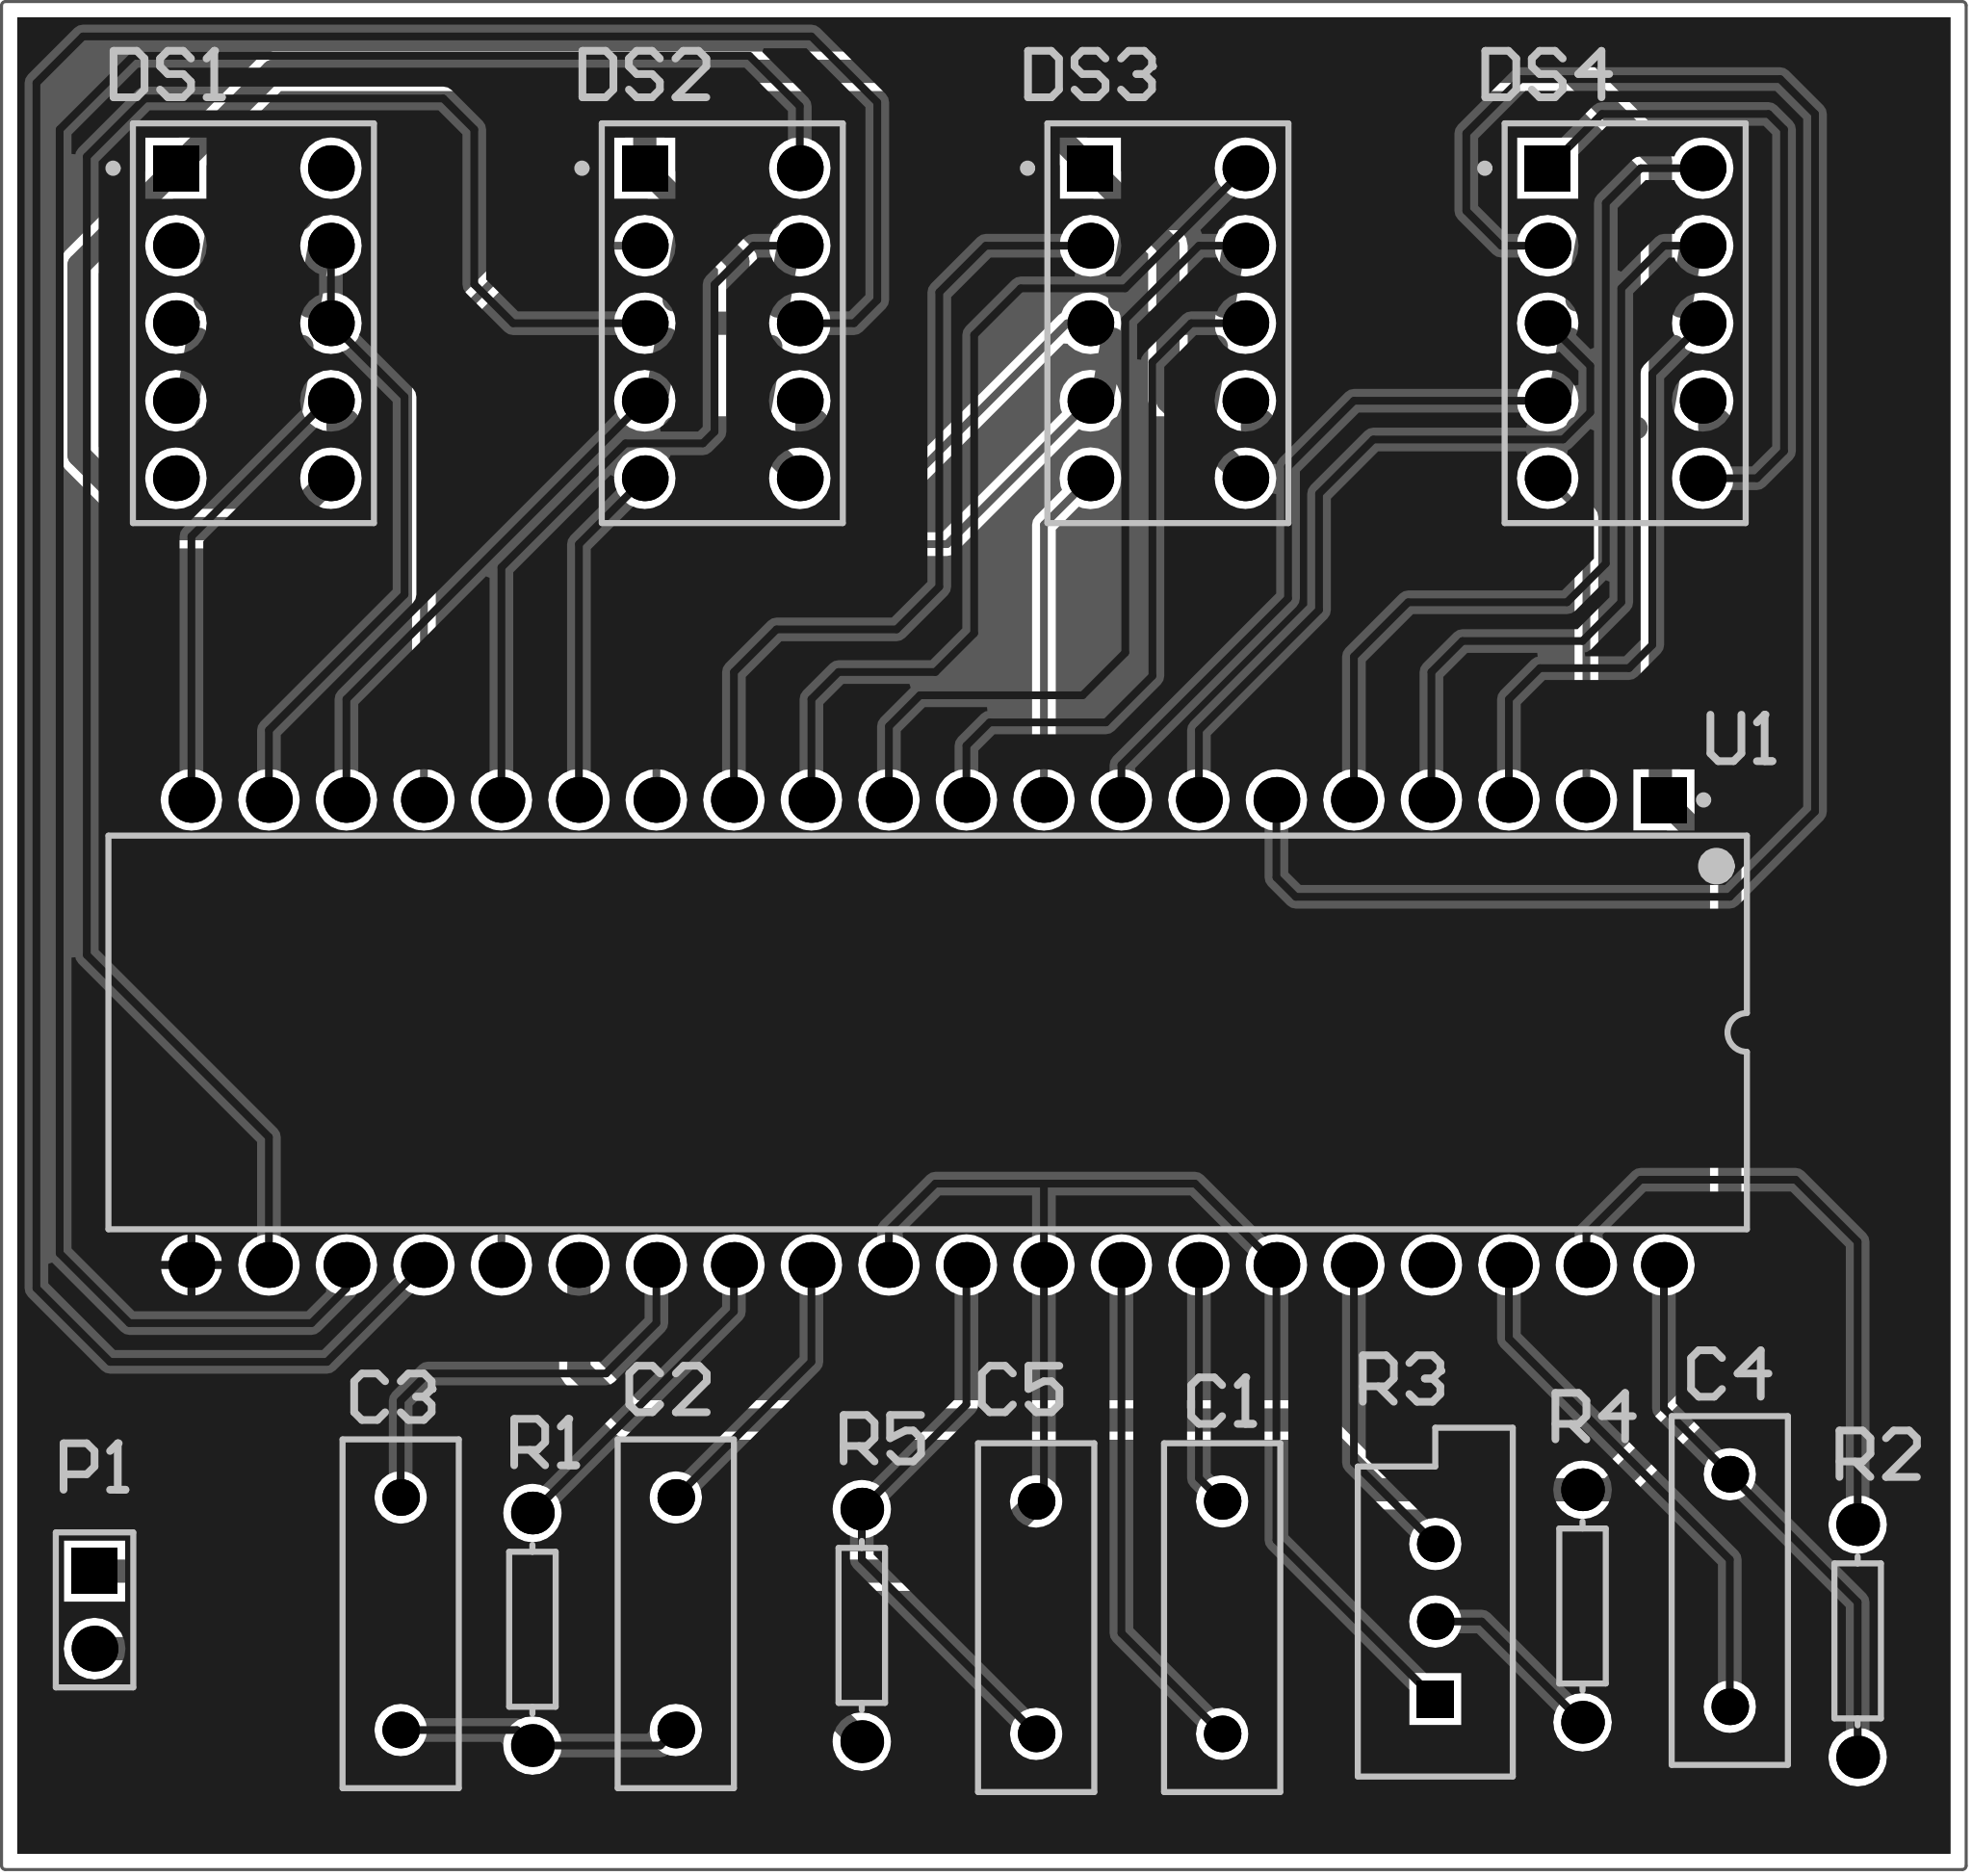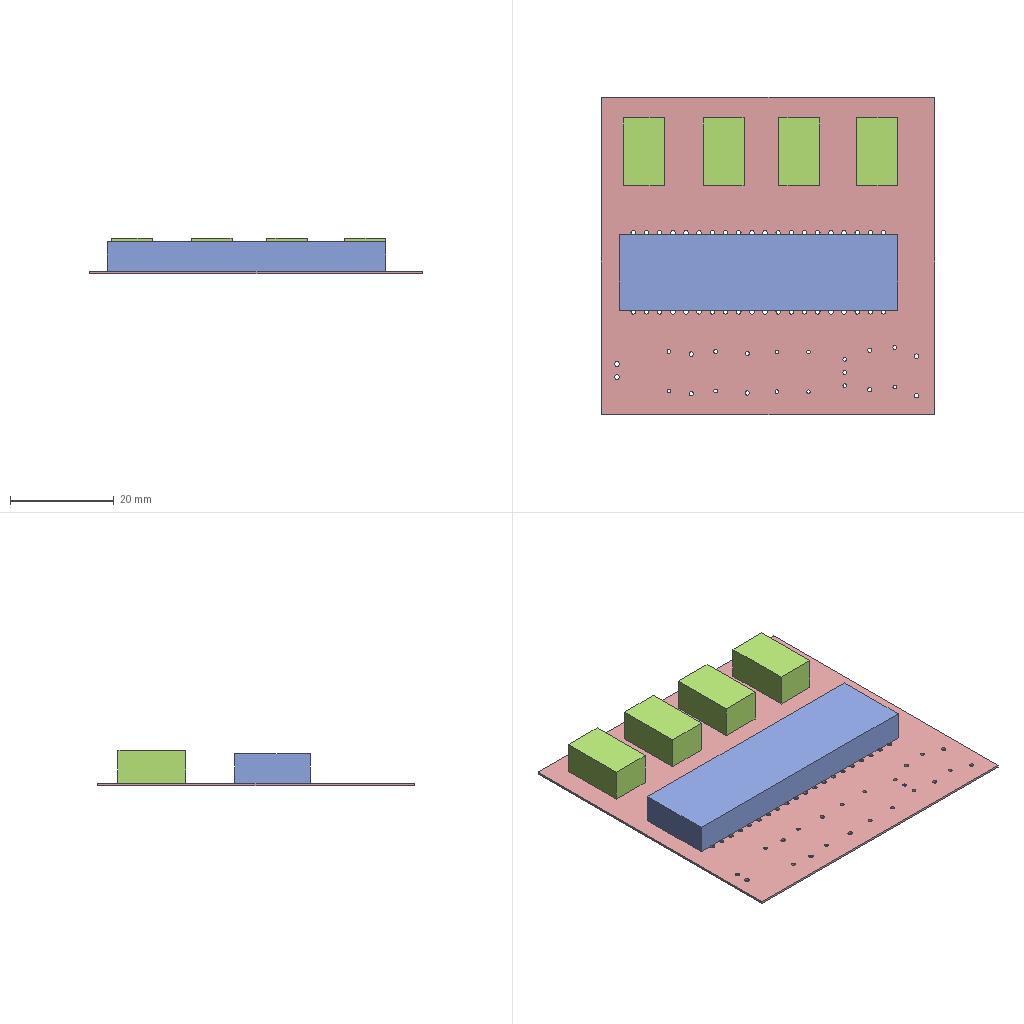Circuit board layout | Altium Designer | box 64.4 x 61.2 x 6.8 mm
Layer stack:
# Altium Designer layer stack of  (unit mm; dielectric type: 0 none, 1 core, 2 prepreg, 3 surface material)
index,name,kind,layer,copper_thickness_mm,dielectric_type,dielectric_thickness_mm,dielectric_material,dielectric_constant
0,Top Paste,other,,,,,,
1,Top Overlay,other,,,,,,
2,Top Solder,dielectric,,,3,0.0102,Solder Resist,3.5
3,Top Layer,copper,Top Layer,0.0356,,,,
4,Dielectric 1,dielectric,,,0,0.32,FR-4,4.8
5,Bottom Layer,copper,Bottom Layer,0.0356,,,,
6,Bottom Solder,dielectric,,,3,0.0102,Solder Resist,3.5
7,Bottom Overlay,other,,,,,,
8,Bottom Paste,other,,,,,,
# drill layer pairs: low layer,high layer
drill_pair,Top Layer,Bottom Layer
Part placement:
Designator,Comment,Layer,Footprint,Center-X(mm),Center-Y(mm),Rotation
U1,ICL7107CJL,TopLayer,JL40A,98.806,66.04,270
R5,1M,TopLayer,AXIAL-0.3,96.647,46.609,90
R4,24K,TopLayer,AXIAL-0.3,120.269,47.244,270
R3,24K,TopLayer,VR5,115.443,46.736,90
R2,100K,TopLayer,AXIAL-0.3,129.286,46.101,90
R1,1M,TopLayer,AXIAL-0.3,85.852,46.482,90
P1,+/-200MV input,TopLayer,HDR1X2,71.501,47.117,270
DS4,Dpy Green-CA,TopLayer,A,121.666,89.281,0
DS3,Dpy Green-CA,TopLayer,A,106.68,89.281,0
DS2,Dpy Green-CA,TopLayer,A,92.075,89.281,0
DS1,Dpy Green-CA,TopLayer,A,76.708,89.281,0
C5,0.02UF,TopLayer,RAD-0.3,102.362,46.863,270
C4,100PF,TopLayer,RAD-0.3,125.095,47.752,90
C3,0.22UF,TopLayer,RAD-0.3,81.534,46.99,270
C2,0.47UF,TopLayer,RAD-0.3,90.551,46.99,270
C1,0.1UF,TopLayer,RAD-0.3,108.458,46.863,270
Pad and via stacks:
# Altium Designer via and pad stacks of  (unit mm). Each distinct definition once, with the count of objects using it.
# via: kind,start_layer,end_layer,hole_mm,diameter_mm,mode(0 simple;1 top-mid-bottom;2 full stack),diameter_per_layer,count,example_net
# pad: kind,layer,hole_mm,hole_type(0 round;1 square;2 slot),plating,top_size,top_shape(1 round;2 rect;3 octagon;9 rounded rect),mid_size,bottom_size,mode,footprint,size_per_layer,count,example
pad,Multi-Layer,0.9,0,plated,1.5x1.5,1,1.5x1.5,1.5x1.5,0,A,,36,DS4.6
pad,Multi-Layer,0.9,0,plated,1.5x1.5,2,1.5x1.5,1.5x1.5,0,A,,4,DS4.1
pad,Multi-Layer,0.9,0,plated,1.5x1.5,1,1.5x1.5,1.5x1.5,0,JL40A,,39,U1.21
pad,Multi-Layer,0.9,0,plated,1.5x1.5,2,1.5x1.5,1.5x1.5,0,JL40A,,1,U1.1
pad,Multi-Layer,0.7,0,plated,1.2x1.2,1,1.2x1.2,1.2x1.2,0,RAD-0.3,,10,C3.2
pad,Multi-Layer,0.85,0,plated,1.4x1.4,1,1.4x1.4,1.4x1.4,0,AXIAL-0.3,,8,R2.2
pad,Multi-Layer,0.7,0,plated,1.2x1.2,2,1.2x1.2,1.2x1.2,0,VR5,,1,R3.1
pad,Multi-Layer,0.7,0,plated,1.2x1.2,1,1.2x1.2,1.2x1.2,0,VR5,,2,R3.2
pad,Multi-Layer,0.9,0,plated,1.5x1.5,2,1.5x1.5,1.5x1.5,0,HDR1X2,,1,P1.1
pad,Multi-Layer,0.9,0,plated,1.5x1.5,1,1.5x1.5,1.5x1.5,0,HDR1X2,,1,P1.2
Copper pours:
name,layer,net,type(0 solid;1 hatched;2 none)
D,Bottom Layer,GND,0
D,Top Layer,GND,0
Design rules, without the lines most boards share:
# Altium Designer design rules of  (exported by Altium Designer, unit mm)
# columns: name | kind | enabled | priority | scope1 | scope2 | descriptor | typed fields (field=value)
SilkToSilkClearance | 55 | enabled | 1 | All | All | Silk to Silk (Clearance=0mil) (All),(All) |
SilkToSolderMaskClearance | 54 | enabled | 1 | IsPad | All | Silk To Solder Mask (Clearance=0mil) (IsPad),(All) |
MinimumSolderMaskSliver | 53 | enabled | 1 | All | All | Minimum Solder Mask Sliver (Gap=0mil) (All),(All) |
HoleToHoleClearance | 52 | enabled | 1 | All | All | Hole To Hole Clearance (Gap=10mil) (All),(All) | gap=0.254
DiffPairsRouting | 51 | enabled | 1 | All | All | Differential Pairs Uncoupled Length using the Gap Constraints (Min=10mil) (Max=10mil) (Prefered=10mil)  and Width Constraints (Min=15mil) (Max=15mil) (Prefered=15mil) (All) |
SolderMaskExpansion | 13 | enabled | 1 | All | All | Solder Mask Expansion (Expansion =4mil) (All) | expansion=0.1016
PasteMaskExpansion | 14 | enabled | 1 | All | All | Paste Mask Expansion (Expansion =0mil) (All) | expansion=0
RoutingVias | 11 | enabled | 1 | All | All | Routing Via (MinHoleWidth=28mil) (MaxHoleWidth=28mil) (PreferredHoleWidth=28mil) (MinWidth=50mil) (MaxWidth=50mil) (PreferedWidth=50mil) (All) | via_min_hole=0.7112 via_max_hole=0.7112 via_preferred_diameter=1.27 via_preferred_hole=0.7112
Width | 2 | enabled | 1 | All | All | Width Constraint (Min=10mil) (Max=30mil) (Preferred=10mil) (All) |
PolygonConnect | 20 | enabled | 1 | All | All | Polygon Connect Rule(Relief Connect )(Conductor Width=10mil) (Relief Angle=90 Angle) (Entries=4) (Air Gap Width=10mil) (All),(All) | connect_style(0=relief,1=direct,2=none)=0 relief_conductor_width=0.254 relief_entries=4
PlaneConnect | 6 | enabled | 1 | All | All | Power Plane Connect Rule(Relief Connect )(Expansion=20mil) (Conductor Width=10mil) (Air Gap=10mil) (Entries=4) (All) | relief_conductor_width=0.254 relief_entries=4 relief_expansion=0.508
Clearance | 0 | enabled | 1 | All | All | Clearance Constraint (Gap=10mil) (All),(All) | gap=0.254
Classes set for this board:
# Altium Designer classes of  (member kind: 0 net, 1 component, 2 from-to, 3 pad, 4 layer, 5 differential pair, 6 design channel, 7 polygon, 8 structure, 9 xSignal)
# columns: class name | member kind | superclass | members
Sheet1 | 1 | no | C1; C2; C3; C4; C5; DS1; DS2; DS3; DS4; P1; R1; R2; R3; R4; R5; U1;